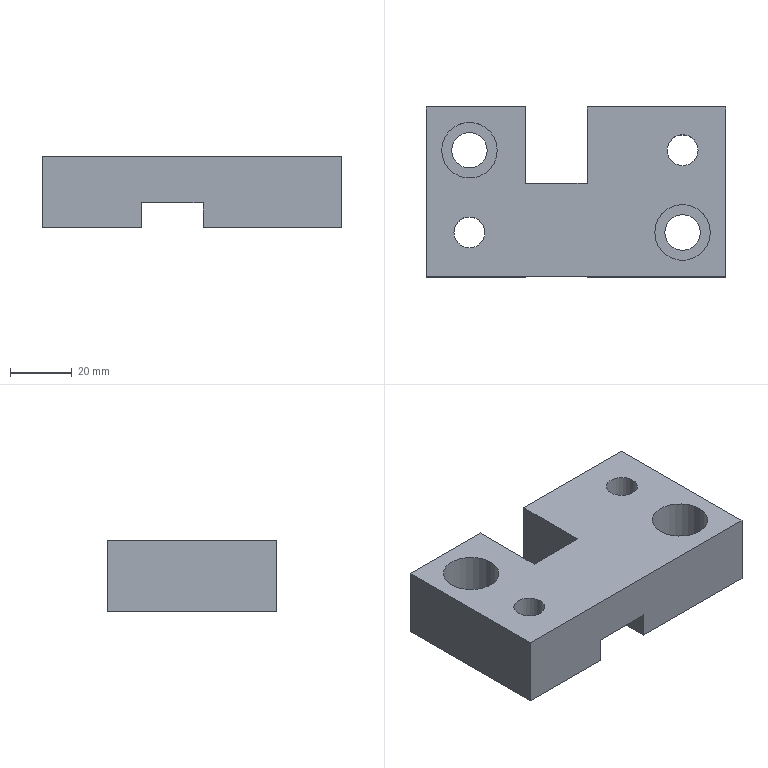Part | STEP file | lll_id4670_x_t | 1 solid | 22 faces | box 97 x 55 x 23 mm | volume 93322 mm3 | plane 15 | cylinder 7 | commonest cylinder face diameters 10 x2 11.509 x2 18.008 x2 8.5 x1
STEP:
#1=CARTESIAN_POINT('',(785.37,-367.421,10.25));
#2=VERTEX_POINT('',#1);
#3=CARTESIAN_POINT('',(785.37,-367.421,14.5));
#4=DIRECTION('',(0.,-1.,0.));
#5=DIRECTION('',(0.,0.,-1.));
#6=AXIS2_PLACEMENT_3D('',#3,#4,#5);
#7=CIRCLE('',#6,4.25);
#8=EDGE_CURVE('',#2,#2,#7,.T.);
#9=ORIENTED_EDGE('',*,*,#8,.T.);
#10=EDGE_LOOP('',(#9));
#11=FACE_BOUND('',#10,.T.);
#12=CARTESIAN_POINT('',(775.37,-367.421,8.));
#13=VERTEX_POINT('',#12);
#14=CARTESIAN_POINT('',(795.37,-367.421,8.));
#15=VERTEX_POINT('',#14);
#16=CARTESIAN_POINT('',(785.37,-367.421,8.));
#17=DIRECTION('',(1.,0.,0.));
#18=VECTOR('',#17,1.);
#19=LINE('',#16,#18);
#20=EDGE_CURVE('',#13,#15,#19,.T.);
#21=ORIENTED_EDGE('',*,*,#20,.F.);
#22=CARTESIAN_POINT('',(775.37,-367.421,23.));
#23=VERTEX_POINT('',#22);
#24=CARTESIAN_POINT('',(775.37,-367.421,12.));
#25=DIRECTION('',(0.,0.,-1.));
#26=VECTOR('',#25,1.);
#27=LINE('',#24,#26);
#28=EDGE_CURVE('',#23,#13,#27,.T.);
#29=ORIENTED_EDGE('',*,*,#28,.F.);
#30=CARTESIAN_POINT('',(795.37,-367.421,23.));
#31=VERTEX_POINT('',#30);
#32=CARTESIAN_POINT('',(785.37,-367.421,23.));
#33=DIRECTION('',(-1.,0.,0.));
#34=VECTOR('',#33,1.);
#35=LINE('',#32,#34);
#36=EDGE_CURVE('',#31,#23,#35,.T.);
#37=ORIENTED_EDGE('',*,*,#36,.F.);
#38=CARTESIAN_POINT('',(795.37,-367.421,12.));
#39=DIRECTION('',(0.,0.,1.));
#40=VECTOR('',#39,1.);
#41=LINE('',#38,#40);
#42=EDGE_CURVE('',#15,#31,#41,.T.);
#43=ORIENTED_EDGE('',*,*,#42,.F.);
#44=EDGE_LOOP('',(#21,#29,#37,#43));
#45=FACE_BOUND('',#44,.T.);
#46=CARTESIAN_POINT('',(785.37,-367.421,12.));
#47=DIRECTION('',(0.,-1.,0.));
#48=DIRECTION('',(0.,0.,-1.));
#49=AXIS2_PLACEMENT_3D('',#46,#47,#48);
#50=PLANE('',#49);
#51=ADVANCED_FACE('',(#11,#45),#50,.F.);
#52=CARTESIAN_POINT('',(762.272,-383.3,23.));
#53=VERTEX_POINT('',#52);
#54=CARTESIAN_POINT('',(757.272,-383.3,23.));
#55=DIRECTION('',(0.,0.,1.));
#56=DIRECTION('',(1.,0.,0.));
#57=AXIS2_PLACEMENT_3D('',#54,#55,#56);
#58=CIRCLE('',#57,5.);
#59=EDGE_CURVE('',#53,#53,#58,.T.);
#60=ORIENTED_EDGE('',*,*,#59,.F.);
#61=EDGE_LOOP('',(#60));
#62=FACE_BOUND('',#61,.T.);
#63=CARTESIAN_POINT('',(835.276,-383.3,23.));
#64=VERTEX_POINT('',#63);
#65=CARTESIAN_POINT('',(826.272,-383.3,23.));
#66=DIRECTION('',(0.,0.,-1.));
#67=DIRECTION('',(1.,0.,0.));
#68=AXIS2_PLACEMENT_3D('',#65,#66,#67);
#69=CIRCLE('',#68,9.004);
#70=EDGE_CURVE('',#64,#64,#69,.T.);
#71=ORIENTED_EDGE('',*,*,#70,.T.);
#72=EDGE_LOOP('',(#71));
#73=FACE_BOUND('',#72,.T.);
#74=CARTESIAN_POINT('',(840.272,-397.7,23.));
#75=VERTEX_POINT('',#74);
#76=CARTESIAN_POINT('',(743.272,-397.7,23.));
#77=VERTEX_POINT('',#76);
#78=CARTESIAN_POINT('',(780.37,-397.7,23.));
#79=DIRECTION('',(-1.,0.,0.));
#80=VECTOR('',#79,1.);
#81=LINE('',#78,#80);
#82=EDGE_CURVE('',#75,#77,#81,.T.);
#83=ORIENTED_EDGE('',*,*,#82,.F.);
#84=CARTESIAN_POINT('',(840.272,-342.7,23.));
#85=VERTEX_POINT('',#84);
#86=CARTESIAN_POINT('',(840.272,-375.96,23.));
#87=DIRECTION('',(0.,1.,0.));
#88=VECTOR('',#87,1.);
#89=LINE('',#86,#88);
#90=EDGE_CURVE('',#75,#85,#89,.T.);
#91=ORIENTED_EDGE('',*,*,#90,.T.);
#92=CARTESIAN_POINT('',(795.37,-342.7,23.));
#93=VERTEX_POINT('',#92);
#94=CARTESIAN_POINT('',(6298.041,-342.7,23.));
#95=DIRECTION('',(1.,0.,0.));
#96=VECTOR('',#95,1.);
#97=LINE('',#94,#96);
#98=EDGE_CURVE('',#93,#85,#97,.T.);
#99=ORIENTED_EDGE('',*,*,#98,.F.);
#100=CARTESIAN_POINT('',(795.37,-341.839,23.));
#101=DIRECTION('',(0.,-1.,0.));
#102=VECTOR('',#101,1.);
#103=LINE('',#100,#102);
#104=EDGE_CURVE('',#93,#31,#103,.T.);
#105=ORIENTED_EDGE('',*,*,#104,.T.);
#106=ORIENTED_EDGE('',*,*,#36,.T.);
#107=CARTESIAN_POINT('',(775.37,-342.7,23.));
#108=VERTEX_POINT('',#107);
#109=CARTESIAN_POINT('',(775.37,-401.921,23.));
#110=DIRECTION('',(0.,1.,0.));
#111=VECTOR('',#110,1.);
#112=LINE('',#109,#111);
#113=EDGE_CURVE('',#23,#108,#112,.T.);
#114=ORIENTED_EDGE('',*,*,#113,.T.);
#115=CARTESIAN_POINT('',(743.272,-342.7,23.));
#116=VERTEX_POINT('',#115);
#117=CARTESIAN_POINT('',(6298.041,-342.7,23.));
#118=DIRECTION('',(1.,0.,0.));
#119=VECTOR('',#118,1.);
#120=LINE('',#117,#119);
#121=EDGE_CURVE('',#116,#108,#120,.T.);
#122=ORIENTED_EDGE('',*,*,#121,.F.);
#123=CARTESIAN_POINT('',(743.272,-381.332,23.));
#124=DIRECTION('',(0.,1.,0.));
#125=VECTOR('',#124,1.);
#126=LINE('',#123,#125);
#127=EDGE_CURVE('',#77,#116,#126,.T.);
#128=ORIENTED_EDGE('',*,*,#127,.F.);
#129=EDGE_LOOP('',(#83,#91,#99,#105,#106,#114,#122,#128));
#130=FACE_BOUND('',#129,.T.);
#131=CARTESIAN_POINT('',(831.272,-356.7,23.));
#132=VERTEX_POINT('',#131);
#133=CARTESIAN_POINT('',(826.272,-356.7,23.));
#134=DIRECTION('',(0.,0.,1.));
#135=DIRECTION('',(1.,0.,0.));
#136=AXIS2_PLACEMENT_3D('',#133,#134,#135);
#137=CIRCLE('',#136,5.);
#138=EDGE_CURVE('',#132,#132,#137,.T.);
#139=ORIENTED_EDGE('',*,*,#138,.F.);
#140=EDGE_LOOP('',(#139));
#141=FACE_BOUND('',#140,.T.);
#142=CARTESIAN_POINT('',(766.276,-356.7,23.));
#143=VERTEX_POINT('',#142);
#144=CARTESIAN_POINT('',(757.272,-356.7,23.));
#145=DIRECTION('',(0.,0.,-1.));
#146=DIRECTION('',(1.,0.,0.));
#147=AXIS2_PLACEMENT_3D('',#144,#145,#146);
#148=CIRCLE('',#147,9.004);
#149=EDGE_CURVE('',#143,#143,#148,.T.);
#150=ORIENTED_EDGE('',*,*,#149,.T.);
#151=EDGE_LOOP('',(#150));
#152=FACE_BOUND('',#151,.T.);
#153=CARTESIAN_POINT('',(780.37,-375.96,23.));
#154=DIRECTION('',(0.,0.,1.));
#155=DIRECTION('',(1.,0.,0.));
#156=AXIS2_PLACEMENT_3D('',#153,#154,#155);
#157=PLANE('',#156);
#158=ADVANCED_FACE('',(#62,#73,#130,#141,#152),#157,.T.);
#159=CARTESIAN_POINT('',(785.37,-382.421,10.25));
#160=VERTEX_POINT('',#159);
#161=CARTESIAN_POINT('',(785.37,-382.421,14.5));
#162=DIRECTION('',(0.,1.,0.));
#163=DIRECTION('',(0.,0.,-1.));
#164=AXIS2_PLACEMENT_3D('',#161,#162,#163);
#165=CIRCLE('',#164,4.25);
#166=EDGE_CURVE('',#160,#160,#165,.T.);
#167=ORIENTED_EDGE('',*,*,#166,.T.);
#168=EDGE_LOOP('',(#167));
#169=FACE_OUTER_BOUND('',#168,.T.);
#170=CARTESIAN_POINT('',(785.37,-382.421,14.5));
#171=DIRECTION('',(0.,-1.,0.));
#172=DIRECTION('',(0.,0.,-1.));
#173=AXIS2_PLACEMENT_3D('',#170,#171,#172);
#174=PLANE('',#173);
#175=ADVANCED_FACE('',(#169),#174,.F.);
#176=CARTESIAN_POINT('',(762.272,-383.3,0.));
#177=VERTEX_POINT('',#176);
#178=CARTESIAN_POINT('',(757.272,-383.3,0.));
#179=DIRECTION('',(0.,0.,1.));
#180=DIRECTION('',(1.,0.,0.));
#181=AXIS2_PLACEMENT_3D('',#178,#179,#180);
#182=CIRCLE('',#181,5.);
#183=EDGE_CURVE('',#177,#177,#182,.T.);
#184=ORIENTED_EDGE('',*,*,#183,.T.);
#185=EDGE_LOOP('',(#184));
#186=FACE_BOUND('',#185,.T.);
#187=CARTESIAN_POINT('',(763.026,-356.7,0.));
#188=VERTEX_POINT('',#187);
#189=CARTESIAN_POINT('',(757.272,-356.7,0.));
#190=DIRECTION('',(0.,0.,1.));
#191=DIRECTION('',(1.,0.,0.));
#192=AXIS2_PLACEMENT_3D('',#189,#190,#191);
#193=CIRCLE('',#192,5.755);
#194=EDGE_CURVE('',#188,#188,#193,.T.);
#195=ORIENTED_EDGE('',*,*,#194,.T.);
#196=EDGE_LOOP('',(#195));
#197=FACE_BOUND('',#196,.T.);
#198=CARTESIAN_POINT('',(775.37,-397.7,0.));
#199=VERTEX_POINT('',#198);
#200=CARTESIAN_POINT('',(775.37,-342.7,0.));
#201=VERTEX_POINT('',#200);
#202=CARTESIAN_POINT('',(775.37,-401.921,0.));
#203=DIRECTION('',(0.,1.,0.));
#204=VECTOR('',#203,1.);
#205=LINE('',#202,#204);
#206=EDGE_CURVE('',#199,#201,#205,.T.);
#207=ORIENTED_EDGE('',*,*,#206,.F.);
#208=CARTESIAN_POINT('',(743.272,-397.7,0.));
#209=VERTEX_POINT('',#208);
#210=CARTESIAN_POINT('',(679.,-397.7,0.));
#211=DIRECTION('',(-1.,0.,0.));
#212=VECTOR('',#211,1.);
#213=LINE('',#210,#212);
#214=EDGE_CURVE('',#199,#209,#213,.T.);
#215=ORIENTED_EDGE('',*,*,#214,.T.);
#216=CARTESIAN_POINT('',(743.272,-342.7,0.));
#217=VERTEX_POINT('',#216);
#218=CARTESIAN_POINT('',(743.272,-381.332,0.));
#219=DIRECTION('',(0.,1.,0.));
#220=VECTOR('',#219,1.);
#221=LINE('',#218,#220);
#222=EDGE_CURVE('',#209,#217,#221,.T.);
#223=ORIENTED_EDGE('',*,*,#222,.T.);
#224=CARTESIAN_POINT('',(6298.041,-342.7,0.));
#225=DIRECTION('',(1.,0.,0.));
#226=VECTOR('',#225,1.);
#227=LINE('',#224,#226);
#228=EDGE_CURVE('',#217,#201,#227,.T.);
#229=ORIENTED_EDGE('',*,*,#228,.T.);
#230=EDGE_LOOP('',(#207,#215,#223,#229));
#231=FACE_BOUND('',#230,.T.);
#232=CARTESIAN_POINT('',(679.,-24.25,0.));
#233=DIRECTION('',(0.,0.,1.));
#234=DIRECTION('',(-1.,0.,0.));
#235=AXIS2_PLACEMENT_3D('',#232,#233,#234);
#236=PLANE('',#235);
#237=ADVANCED_FACE('',(#186,#197,#231),#236,.F.);
#238=CARTESIAN_POINT('',(831.272,-356.7,0.));
#239=VERTEX_POINT('',#238);
#240=CARTESIAN_POINT('',(826.272,-356.7,0.));
#241=DIRECTION('',(0.,0.,1.));
#242=DIRECTION('',(1.,0.,0.));
#243=AXIS2_PLACEMENT_3D('',#240,#241,#242);
#244=CIRCLE('',#243,5.);
#245=EDGE_CURVE('',#239,#239,#244,.T.);
#246=ORIENTED_EDGE('',*,*,#245,.T.);
#247=EDGE_LOOP('',(#246));
#248=FACE_BOUND('',#247,.T.);
#249=CARTESIAN_POINT('',(832.026,-383.3,0.));
#250=VERTEX_POINT('',#249);
#251=CARTESIAN_POINT('',(826.272,-383.3,0.));
#252=DIRECTION('',(0.,0.,1.));
#253=DIRECTION('',(1.,0.,0.));
#254=AXIS2_PLACEMENT_3D('',#251,#252,#253);
#255=CIRCLE('',#254,5.755);
#256=EDGE_CURVE('',#250,#250,#255,.T.);
#257=ORIENTED_EDGE('',*,*,#256,.T.);
#258=EDGE_LOOP('',(#257));
#259=FACE_BOUND('',#258,.T.);
#260=CARTESIAN_POINT('',(840.272,-342.7,0.));
#261=VERTEX_POINT('',#260);
#262=CARTESIAN_POINT('',(840.272,-397.7,0.));
#263=VERTEX_POINT('',#262);
#264=CARTESIAN_POINT('',(840.272,-381.332,0.));
#265=DIRECTION('',(0.,-1.,0.));
#266=VECTOR('',#265,1.);
#267=LINE('',#264,#266);
#268=EDGE_CURVE('',#261,#263,#267,.T.);
#269=ORIENTED_EDGE('',*,*,#268,.T.);
#270=CARTESIAN_POINT('',(795.37,-397.7,0.));
#271=VERTEX_POINT('',#270);
#272=CARTESIAN_POINT('',(679.,-397.7,0.));
#273=DIRECTION('',(-1.,0.,0.));
#274=VECTOR('',#273,1.);
#275=LINE('',#272,#274);
#276=EDGE_CURVE('',#263,#271,#275,.T.);
#277=ORIENTED_EDGE('',*,*,#276,.T.);
#278=CARTESIAN_POINT('',(795.37,-342.7,0.));
#279=VERTEX_POINT('',#278);
#280=CARTESIAN_POINT('',(795.37,-341.839,0.));
#281=DIRECTION('',(0.,-1.,0.));
#282=VECTOR('',#281,1.);
#283=LINE('',#280,#282);
#284=EDGE_CURVE('',#279,#271,#283,.T.);
#285=ORIENTED_EDGE('',*,*,#284,.F.);
#286=CARTESIAN_POINT('',(6298.041,-342.7,0.));
#287=DIRECTION('',(1.,0.,0.));
#288=VECTOR('',#287,1.);
#289=LINE('',#286,#288);
#290=EDGE_CURVE('',#279,#261,#289,.T.);
#291=ORIENTED_EDGE('',*,*,#290,.T.);
#292=EDGE_LOOP('',(#269,#277,#285,#291));
#293=FACE_BOUND('',#292,.T.);
#294=CARTESIAN_POINT('',(679.,-24.25,0.));
#295=DIRECTION('',(0.,0.,1.));
#296=DIRECTION('',(-1.,0.,0.));
#297=AXIS2_PLACEMENT_3D('',#294,#295,#296);
#298=PLANE('',#297);
#299=ADVANCED_FACE('',(#248,#259,#293),#298,.F.);
#300=CARTESIAN_POINT('',(775.37,-342.7,2.5));
#301=DIRECTION('',(0.,0.,1.));
#302=VECTOR('',#301,1.);
#303=LINE('',#300,#302);
#304=EDGE_CURVE('',#201,#108,#303,.T.);
#305=ORIENTED_EDGE('',*,*,#304,.F.);
#306=ORIENTED_EDGE('',*,*,#228,.F.);
#307=CARTESIAN_POINT('',(743.272,-342.7,2.5));
#308=DIRECTION('',(0.,0.,1.));
#309=VECTOR('',#308,1.);
#310=LINE('',#307,#309);
#311=EDGE_CURVE('',#217,#116,#310,.T.);
#312=ORIENTED_EDGE('',*,*,#311,.T.);
#313=ORIENTED_EDGE('',*,*,#121,.T.);
#314=EDGE_LOOP('',(#305,#306,#312,#313));
#315=FACE_OUTER_BOUND('',#314,.T.);
#316=CARTESIAN_POINT('',(6298.041,-342.7,2.5));
#317=DIRECTION('',(0.,-1.,0.));
#318=DIRECTION('',(0.,0.,-1.));
#319=AXIS2_PLACEMENT_3D('',#316,#317,#318);
#320=PLANE('',#319);
#321=ADVANCED_FACE('',(#315),#320,.F.);
#322=CARTESIAN_POINT('',(795.37,-342.7,2.5));
#323=DIRECTION('',(0.,0.,-1.));
#324=VECTOR('',#323,1.);
#325=LINE('',#322,#324);
#326=EDGE_CURVE('',#93,#279,#325,.T.);
#327=ORIENTED_EDGE('',*,*,#326,.F.);
#328=ORIENTED_EDGE('',*,*,#98,.T.);
#329=CARTESIAN_POINT('',(840.272,-342.7,-10.));
#330=DIRECTION('',(0.,0.,1.));
#331=VECTOR('',#330,1.);
#332=LINE('',#329,#331);
#333=EDGE_CURVE('',#261,#85,#332,.T.);
#334=ORIENTED_EDGE('',*,*,#333,.F.);
#335=ORIENTED_EDGE('',*,*,#290,.F.);
#336=EDGE_LOOP('',(#327,#328,#334,#335));
#337=FACE_OUTER_BOUND('',#336,.T.);
#338=CARTESIAN_POINT('',(6298.041,-342.7,2.5));
#339=DIRECTION('',(0.,-1.,0.));
#340=DIRECTION('',(0.,0.,-1.));
#341=AXIS2_PLACEMENT_3D('',#338,#339,#340);
#342=PLANE('',#341);
#343=ADVANCED_FACE('',(#337),#342,.F.);
#344=CARTESIAN_POINT('',(840.272,-397.7,11.5));
#345=DIRECTION('',(0.,0.,-1.));
#346=VECTOR('',#345,1.);
#347=LINE('',#344,#346);
#348=EDGE_CURVE('',#75,#263,#347,.T.);
#349=ORIENTED_EDGE('',*,*,#348,.T.);
#350=ORIENTED_EDGE('',*,*,#268,.F.);
#351=ORIENTED_EDGE('',*,*,#333,.T.);
#352=ORIENTED_EDGE('',*,*,#90,.F.);
#353=EDGE_LOOP('',(#349,#350,#351,#352));
#354=FACE_OUTER_BOUND('',#353,.T.);
#355=CARTESIAN_POINT('',(840.272,-381.332,-10.));
#356=DIRECTION('',(1.,0.,0.));
#357=DIRECTION('',(0.,0.,1.));
#358=AXIS2_PLACEMENT_3D('',#355,#356,#357);
#359=PLANE('',#358);
#360=ADVANCED_FACE('',(#354),#359,.T.);
#361=CARTESIAN_POINT('',(743.272,-397.7,11.5));
#362=DIRECTION('',(0.,0.,1.));
#363=VECTOR('',#362,1.);
#364=LINE('',#361,#363);
#365=EDGE_CURVE('',#209,#77,#364,.T.);
#366=ORIENTED_EDGE('',*,*,#365,.T.);
#367=ORIENTED_EDGE('',*,*,#127,.T.);
#368=ORIENTED_EDGE('',*,*,#311,.F.);
#369=ORIENTED_EDGE('',*,*,#222,.F.);
#370=EDGE_LOOP('',(#366,#367,#368,#369));
#371=FACE_OUTER_BOUND('',#370,.T.);
#372=CARTESIAN_POINT('',(743.272,-381.332,-10.));
#373=DIRECTION('',(-1.,0.,0.));
#374=DIRECTION('',(0.,0.,-1.));
#375=AXIS2_PLACEMENT_3D('',#372,#373,#374);
#376=PLANE('',#375);
#377=ADVANCED_FACE('',(#371),#376,.T.);
#378=CARTESIAN_POINT('',(775.37,-397.7,8.));
#379=VERTEX_POINT('',#378);
#380=CARTESIAN_POINT('',(775.37,-379.291,8.));
#381=DIRECTION('',(0.,1.,0.));
#382=VECTOR('',#381,1.);
#383=LINE('',#380,#382);
#384=EDGE_CURVE('',#379,#13,#383,.T.);
#385=ORIENTED_EDGE('',*,*,#384,.F.);
#386=CARTESIAN_POINT('',(775.37,-397.7,11.5));
#387=DIRECTION('',(0.,0.,1.));
#388=VECTOR('',#387,1.);
#389=LINE('',#386,#388);
#390=EDGE_CURVE('',#199,#379,#389,.T.);
#391=ORIENTED_EDGE('',*,*,#390,.F.);
#392=ORIENTED_EDGE('',*,*,#206,.T.);
#393=ORIENTED_EDGE('',*,*,#304,.T.);
#394=ORIENTED_EDGE('',*,*,#113,.F.);
#395=ORIENTED_EDGE('',*,*,#28,.T.);
#396=EDGE_LOOP('',(#385,#391,#392,#393,#394,#395));
#397=FACE_OUTER_BOUND('',#396,.T.);
#398=CARTESIAN_POINT('',(775.37,-401.921,-2.));
#399=DIRECTION('',(-1.,0.,0.));
#400=DIRECTION('',(0.,0.,1.));
#401=AXIS2_PLACEMENT_3D('',#398,#399,#400);
#402=PLANE('',#401);
#403=ADVANCED_FACE('',(#397),#402,.F.);
#404=ORIENTED_EDGE('',*,*,#326,.T.);
#405=ORIENTED_EDGE('',*,*,#284,.T.);
#406=CARTESIAN_POINT('',(795.37,-397.7,8.));
#407=VERTEX_POINT('',#406);
#408=CARTESIAN_POINT('',(795.37,-397.7,-2.));
#409=DIRECTION('',(0.,0.,1.));
#410=VECTOR('',#409,1.);
#411=LINE('',#408,#410);
#412=EDGE_CURVE('',#271,#407,#411,.T.);
#413=ORIENTED_EDGE('',*,*,#412,.T.);
#414=CARTESIAN_POINT('',(795.37,-379.291,8.));
#415=DIRECTION('',(0.,-1.,0.));
#416=VECTOR('',#415,1.);
#417=LINE('',#414,#416);
#418=EDGE_CURVE('',#15,#407,#417,.T.);
#419=ORIENTED_EDGE('',*,*,#418,.F.);
#420=ORIENTED_EDGE('',*,*,#42,.T.);
#421=ORIENTED_EDGE('',*,*,#104,.F.);
#422=EDGE_LOOP('',(#404,#405,#413,#419,#420,#421));
#423=FACE_OUTER_BOUND('',#422,.T.);
#424=CARTESIAN_POINT('',(795.37,-341.839,-2.));
#425=DIRECTION('',(1.,0.,0.));
#426=DIRECTION('',(0.,0.,-1.));
#427=AXIS2_PLACEMENT_3D('',#424,#425,#426);
#428=PLANE('',#427);
#429=ADVANCED_FACE('',(#423),#428,.F.);
#430=ORIENTED_EDGE('',*,*,#166,.F.);
#431=EDGE_LOOP('',(#430));
#432=FACE_BOUND('',#431,.T.);
#433=ORIENTED_EDGE('',*,*,#8,.F.);
#434=EDGE_LOOP('',(#433));
#435=FACE_BOUND('',#434,.T.);
#436=CARTESIAN_POINT('',(785.37,-371.921,14.5));
#437=DIRECTION('',(0.,-1.,0.));
#438=DIRECTION('',(0.,0.,-1.));
#439=AXIS2_PLACEMENT_3D('',#436,#437,#438);
#440=CYLINDRICAL_SURFACE('',#439,4.25);
#441=ADVANCED_FACE('',(#432,#435),#440,.F.);
#442=CARTESIAN_POINT('',(817.821,-397.7,8.));
#443=DIRECTION('',(1.,0.,0.));
#444=VECTOR('',#443,1.);
#445=LINE('',#442,#444);
#446=EDGE_CURVE('',#379,#407,#445,.T.);
#447=ORIENTED_EDGE('',*,*,#446,.T.);
#448=ORIENTED_EDGE('',*,*,#412,.F.);
#449=ORIENTED_EDGE('',*,*,#276,.F.);
#450=ORIENTED_EDGE('',*,*,#348,.F.);
#451=ORIENTED_EDGE('',*,*,#82,.T.);
#452=ORIENTED_EDGE('',*,*,#365,.F.);
#453=ORIENTED_EDGE('',*,*,#214,.F.);
#454=ORIENTED_EDGE('',*,*,#390,.T.);
#455=EDGE_LOOP('',(#447,#448,#449,#450,#451,#452,#453,#454));
#456=FACE_OUTER_BOUND('',#455,.T.);
#457=CARTESIAN_POINT('',(817.821,-397.7,11.5));
#458=DIRECTION('',(0.,1.,0.));
#459=DIRECTION('',(0.,0.,1.));
#460=AXIS2_PLACEMENT_3D('',#457,#458,#459);
#461=PLANE('',#460);
#462=ADVANCED_FACE('',(#456),#461,.F.);
#463=CARTESIAN_POINT('',(820.517,-383.3,10.));
#464=VERTEX_POINT('',#463);
#465=CARTESIAN_POINT('',(826.272,-383.3,10.));
#466=DIRECTION('',(0.,0.,-1.));
#467=DIRECTION('',(-1.,0.,0.));
#468=AXIS2_PLACEMENT_3D('',#465,#466,#467);
#469=CIRCLE('',#468,5.755);
#470=EDGE_CURVE('',#464,#464,#469,.T.);
#471=ORIENTED_EDGE('',*,*,#470,.F.);
#472=EDGE_LOOP('',(#471));
#473=FACE_BOUND('',#472,.T.);
#474=ORIENTED_EDGE('',*,*,#256,.F.);
#475=EDGE_LOOP('',(#474));
#476=FACE_BOUND('',#475,.T.);
#477=CARTESIAN_POINT('',(826.272,-383.3,25.));
#478=DIRECTION('',(0.,0.,-1.));
#479=DIRECTION('',(1.,0.,0.));
#480=AXIS2_PLACEMENT_3D('',#477,#478,#479);
#481=CYLINDRICAL_SURFACE('',#480,5.755);
#482=ADVANCED_FACE('',(#473,#476),#481,.F.);
#483=ORIENTED_EDGE('',*,*,#470,.T.);
#484=EDGE_LOOP('',(#483));
#485=FACE_BOUND('',#484,.T.);
#486=CARTESIAN_POINT('',(835.276,-383.3,10.));
#487=VERTEX_POINT('',#486);
#488=CARTESIAN_POINT('',(826.272,-383.3,10.));
#489=DIRECTION('',(0.,0.,-1.));
#490=DIRECTION('',(1.,0.,0.));
#491=AXIS2_PLACEMENT_3D('',#488,#489,#490);
#492=CIRCLE('',#491,9.004);
#493=EDGE_CURVE('',#487,#487,#492,.T.);
#494=ORIENTED_EDGE('',*,*,#493,.F.);
#495=EDGE_LOOP('',(#494));
#496=FACE_BOUND('',#495,.T.);
#497=CARTESIAN_POINT('',(826.272,-383.3,10.));
#498=DIRECTION('',(0.,0.,-1.));
#499=DIRECTION('',(-1.,0.,0.));
#500=AXIS2_PLACEMENT_3D('',#497,#498,#499);
#501=PLANE('',#500);
#502=ADVANCED_FACE('',(#485,#496),#501,.F.);
#503=ORIENTED_EDGE('',*,*,#493,.T.);
#504=EDGE_LOOP('',(#503));
#505=FACE_BOUND('',#504,.T.);
#506=ORIENTED_EDGE('',*,*,#70,.F.);
#507=EDGE_LOOP('',(#506));
#508=FACE_BOUND('',#507,.T.);
#509=CARTESIAN_POINT('',(826.272,-383.3,23.));
#510=DIRECTION('',(0.,0.,-1.));
#511=DIRECTION('',(1.,0.,0.));
#512=AXIS2_PLACEMENT_3D('',#509,#510,#511);
#513=CYLINDRICAL_SURFACE('',#512,9.004);
#514=ADVANCED_FACE('',(#505,#508),#513,.F.);
#515=ORIENTED_EDGE('',*,*,#138,.T.);
#516=EDGE_LOOP('',(#515));
#517=FACE_BOUND('',#516,.T.);
#518=ORIENTED_EDGE('',*,*,#245,.F.);
#519=EDGE_LOOP('',(#518));
#520=FACE_BOUND('',#519,.T.);
#521=CARTESIAN_POINT('',(826.272,-356.7,25.));
#522=DIRECTION('',(0.,0.,-1.));
#523=DIRECTION('',(1.,0.,0.));
#524=AXIS2_PLACEMENT_3D('',#521,#522,#523);
#525=CYLINDRICAL_SURFACE('',#524,5.);
#526=ADVANCED_FACE('',(#517,#520),#525,.F.);
#527=CARTESIAN_POINT('',(751.517,-356.7,10.));
#528=VERTEX_POINT('',#527);
#529=CARTESIAN_POINT('',(757.272,-356.7,10.));
#530=DIRECTION('',(0.,0.,-1.));
#531=DIRECTION('',(-1.,0.,0.));
#532=AXIS2_PLACEMENT_3D('',#529,#530,#531);
#533=CIRCLE('',#532,5.755);
#534=EDGE_CURVE('',#528,#528,#533,.T.);
#535=ORIENTED_EDGE('',*,*,#534,.F.);
#536=EDGE_LOOP('',(#535));
#537=FACE_BOUND('',#536,.T.);
#538=ORIENTED_EDGE('',*,*,#194,.F.);
#539=EDGE_LOOP('',(#538));
#540=FACE_BOUND('',#539,.T.);
#541=CARTESIAN_POINT('',(757.272,-356.7,25.));
#542=DIRECTION('',(0.,0.,-1.));
#543=DIRECTION('',(1.,0.,0.));
#544=AXIS2_PLACEMENT_3D('',#541,#542,#543);
#545=CYLINDRICAL_SURFACE('',#544,5.755);
#546=ADVANCED_FACE('',(#537,#540),#545,.F.);
#547=ORIENTED_EDGE('',*,*,#534,.T.);
#548=EDGE_LOOP('',(#547));
#549=FACE_BOUND('',#548,.T.);
#550=CARTESIAN_POINT('',(766.276,-356.7,10.));
#551=VERTEX_POINT('',#550);
#552=CARTESIAN_POINT('',(757.272,-356.7,10.));
#553=DIRECTION('',(0.,0.,-1.));
#554=DIRECTION('',(1.,0.,0.));
#555=AXIS2_PLACEMENT_3D('',#552,#553,#554);
#556=CIRCLE('',#555,9.004);
#557=EDGE_CURVE('',#551,#551,#556,.T.);
#558=ORIENTED_EDGE('',*,*,#557,.F.);
#559=EDGE_LOOP('',(#558));
#560=FACE_BOUND('',#559,.T.);
#561=CARTESIAN_POINT('',(757.272,-356.7,10.));
#562=DIRECTION('',(0.,0.,-1.));
#563=DIRECTION('',(-1.,0.,0.));
#564=AXIS2_PLACEMENT_3D('',#561,#562,#563);
#565=PLANE('',#564);
#566=ADVANCED_FACE('',(#549,#560),#565,.F.);
#567=ORIENTED_EDGE('',*,*,#557,.T.);
#568=EDGE_LOOP('',(#567));
#569=FACE_BOUND('',#568,.T.);
#570=ORIENTED_EDGE('',*,*,#149,.F.);
#571=EDGE_LOOP('',(#570));
#572=FACE_BOUND('',#571,.T.);
#573=CARTESIAN_POINT('',(757.272,-356.7,23.));
#574=DIRECTION('',(0.,0.,-1.));
#575=DIRECTION('',(1.,0.,0.));
#576=AXIS2_PLACEMENT_3D('',#573,#574,#575);
#577=CYLINDRICAL_SURFACE('',#576,9.004);
#578=ADVANCED_FACE('',(#569,#572),#577,.F.);
#579=ORIENTED_EDGE('',*,*,#59,.T.);
#580=EDGE_LOOP('',(#579));
#581=FACE_BOUND('',#580,.T.);
#582=ORIENTED_EDGE('',*,*,#183,.F.);
#583=EDGE_LOOP('',(#582));
#584=FACE_BOUND('',#583,.T.);
#585=CARTESIAN_POINT('',(757.272,-383.3,25.));
#586=DIRECTION('',(0.,0.,-1.));
#587=DIRECTION('',(1.,0.,0.));
#588=AXIS2_PLACEMENT_3D('',#585,#586,#587);
#589=CYLINDRICAL_SURFACE('',#588,5.);
#590=ADVANCED_FACE('',(#581,#584),#589,.F.);
#591=ORIENTED_EDGE('',*,*,#20,.T.);
#592=ORIENTED_EDGE('',*,*,#418,.T.);
#593=ORIENTED_EDGE('',*,*,#446,.F.);
#594=ORIENTED_EDGE('',*,*,#384,.T.);
#595=EDGE_LOOP('',(#591,#592,#593,#594));
#596=FACE_OUTER_BOUND('',#595,.T.);
#597=CARTESIAN_POINT('',(785.37,-379.291,8.));
#598=DIRECTION('',(0.,0.,-1.));
#599=DIRECTION('',(-1.,0.,0.));
#600=AXIS2_PLACEMENT_3D('',#597,#598,#599);
#601=PLANE('',#600);
#602=ADVANCED_FACE('',(#596),#601,.T.);
#603=CLOSED_SHELL('',(#51,#158,#175,#237,#299,#321,#343,#360,#377,#403,#429,#441,#462,#482,#502,#514,#526,#546,#566,#578,#590,#602));
#604=MANIFOLD_SOLID_BREP('',#603);
#605=(LENGTH_UNIT()NAMED_UNIT(*)SI_UNIT(.MILLI.,.METRE.));
#606=UNCERTAINTY_MEASURE_WITH_UNIT(LENGTH_MEASURE(0.00002),#605,'','');
#607=(NAMED_UNIT(*)PLANE_ANGLE_UNIT()SI_UNIT($,.RADIAN.));
#608=PLANE_ANGLE_MEASURE_WITH_UNIT(PLANE_ANGLE_MEASURE(0.01745),#607);
#609=DIMENSIONAL_EXPONENTS(0.,0.,0.,0.,0.,0.,0.);
#610=(CONVERSION_BASED_UNIT('DEGREE',#608)NAMED_UNIT(#609)PLANE_ANGLE_UNIT());
#611=(NAMED_UNIT(*)SI_UNIT($,.STERADIAN.)SOLID_ANGLE_UNIT());
#612=(GEOMETRIC_REPRESENTATION_CONTEXT(3)GLOBAL_UNCERTAINTY_ASSIGNED_CONTEXT((#606))GLOBAL_UNIT_ASSIGNED_CONTEXT((#605,#610,#611))REPRESENTATION_CONTEXT('',''));
#613=ADVANCED_BREP_SHAPE_REPRESENTATION('',(#604),#612);